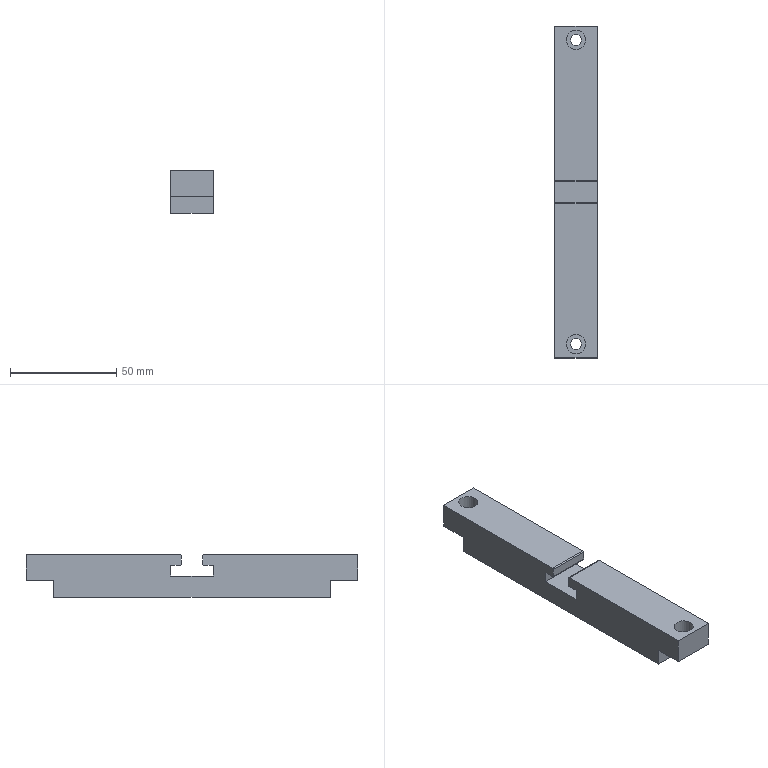Part | STEP file | 200 mesh_id1914 | 1 solid | 28 faces | box 20 x 156 x 20 mm | volume 54101 mm3 | plane 20 | cylinder 8 | commonest cylinder face diameters 1 x4 5.2 x2 9 x2
STEP:
#1=CARTESIAN_POINT('',(-16722.684,-4085.169,68.43));
#2=VERTEX_POINT('',#1);
#3=CARTESIAN_POINT('',(-16722.684,-4098.269,68.43));
#4=VERTEX_POINT('',#3);
#5=CARTESIAN_POINT('',(-16722.684,-4095.569,68.43));
#6=DIRECTION('',(0.,-1.,0.));
#7=VECTOR('',#6,1.);
#8=LINE('',#5,#7);
#9=EDGE_CURVE('',#2,#4,#8,.T.);
#10=ORIENTED_EDGE('',*,*,#9,.F.);
#11=CARTESIAN_POINT('',(-16722.684,-4085.169,60.43));
#12=VERTEX_POINT('',#11);
#13=CARTESIAN_POINT('',(-16722.684,-4085.169,68.63));
#14=DIRECTION('',(0.,0.,-1.));
#15=VECTOR('',#14,1.);
#16=LINE('',#13,#15);
#17=EDGE_CURVE('',#2,#12,#16,.T.);
#18=ORIENTED_EDGE('',*,*,#17,.T.);
#19=CARTESIAN_POINT('',(-16722.684,-3955.369,60.43));
#20=VERTEX_POINT('',#19);
#21=CARTESIAN_POINT('',(-16722.684,-4095.269,60.43));
#22=DIRECTION('',(0.,1.,0.));
#23=VECTOR('',#22,1.);
#24=LINE('',#21,#23);
#25=EDGE_CURVE('',#12,#20,#24,.T.);
#26=ORIENTED_EDGE('',*,*,#25,.T.);
#27=CARTESIAN_POINT('',(-16722.684,-3955.369,68.43));
#28=VERTEX_POINT('',#27);
#29=CARTESIAN_POINT('',(-16722.684,-3955.369,68.63));
#30=DIRECTION('',(0.,0.,1.));
#31=VECTOR('',#30,1.);
#32=LINE('',#29,#31);
#33=EDGE_CURVE('',#20,#28,#32,.T.);
#34=ORIENTED_EDGE('',*,*,#33,.T.);
#35=CARTESIAN_POINT('',(-16722.684,-3942.269,68.43));
#36=VERTEX_POINT('',#35);
#37=CARTESIAN_POINT('',(-16722.684,-3955.369,68.43));
#38=DIRECTION('',(0.,1.,0.));
#39=VECTOR('',#38,1.);
#40=LINE('',#37,#39);
#41=EDGE_CURVE('',#28,#36,#40,.T.);
#42=ORIENTED_EDGE('',*,*,#41,.T.);
#43=CARTESIAN_POINT('',(-16722.684,-3942.269,80.43));
#44=VERTEX_POINT('',#43);
#45=CARTESIAN_POINT('',(-16722.684,-3942.269,60.186));
#46=DIRECTION('',(0.,0.,1.));
#47=VECTOR('',#46,1.);
#48=LINE('',#45,#47);
#49=EDGE_CURVE('',#36,#44,#48,.T.);
#50=ORIENTED_EDGE('',*,*,#49,.T.);
#51=CARTESIAN_POINT('',(-16722.684,-4014.769,80.43));
#52=VERTEX_POINT('',#51);
#53=CARTESIAN_POINT('',(-16722.684,-4095.269,80.43));
#54=DIRECTION('',(0.,1.,0.));
#55=VECTOR('',#54,1.);
#56=LINE('',#53,#55);
#57=EDGE_CURVE('',#52,#44,#56,.T.);
#58=ORIENTED_EDGE('',*,*,#57,.F.);
#59=CARTESIAN_POINT('',(-16722.684,-4015.269,79.93));
#60=VERTEX_POINT('',#59);
#61=CARTESIAN_POINT('',(-16722.684,-4014.769,79.93));
#62=DIRECTION('',(1.,0.,0.));
#63=DIRECTION('',(0.,1.,0.));
#64=AXIS2_PLACEMENT_3D('',#61,#62,#63);
#65=CIRCLE('',#64,0.5);
#66=EDGE_CURVE('',#52,#60,#65,.T.);
#67=ORIENTED_EDGE('',*,*,#66,.T.);
#68=CARTESIAN_POINT('',(-16722.684,-4015.269,75.93));
#69=VERTEX_POINT('',#68);
#70=CARTESIAN_POINT('',(-16722.684,-4015.269,80.43));
#71=DIRECTION('',(0.,0.,-1.));
#72=VECTOR('',#71,1.);
#73=LINE('',#70,#72);
#74=EDGE_CURVE('',#60,#69,#73,.T.);
#75=ORIENTED_EDGE('',*,*,#74,.T.);
#76=CARTESIAN_POINT('',(-16722.684,-4014.769,75.43));
#77=VERTEX_POINT('',#76);
#78=CARTESIAN_POINT('',(-16722.684,-4014.769,75.93));
#79=DIRECTION('',(1.,0.,0.));
#80=DIRECTION('',(0.,1.,0.));
#81=AXIS2_PLACEMENT_3D('',#78,#79,#80);
#82=CIRCLE('',#81,0.5);
#83=EDGE_CURVE('',#69,#77,#82,.T.);
#84=ORIENTED_EDGE('',*,*,#83,.T.);
#85=CARTESIAN_POINT('',(-16722.684,-4010.269,75.43));
#86=VERTEX_POINT('',#85);
#87=CARTESIAN_POINT('',(-16722.684,-4015.269,75.43));
#88=DIRECTION('',(0.,1.,0.));
#89=VECTOR('',#88,1.);
#90=LINE('',#87,#89);
#91=EDGE_CURVE('',#77,#86,#90,.T.);
#92=ORIENTED_EDGE('',*,*,#91,.T.);
#93=CARTESIAN_POINT('',(-16722.684,-4010.269,70.43));
#94=VERTEX_POINT('',#93);
#95=CARTESIAN_POINT('',(-16722.684,-4010.269,75.43));
#96=DIRECTION('',(0.,0.,-1.));
#97=VECTOR('',#96,1.);
#98=LINE('',#95,#97);
#99=EDGE_CURVE('',#86,#94,#98,.T.);
#100=ORIENTED_EDGE('',*,*,#99,.T.);
#101=CARTESIAN_POINT('',(-16722.684,-4030.269,70.43));
#102=VERTEX_POINT('',#101);
#103=CARTESIAN_POINT('',(-16722.684,-4010.269,70.43));
#104=DIRECTION('',(0.,-1.,0.));
#105=VECTOR('',#104,1.);
#106=LINE('',#103,#105);
#107=EDGE_CURVE('',#94,#102,#106,.T.);
#108=ORIENTED_EDGE('',*,*,#107,.T.);
#109=CARTESIAN_POINT('',(-16722.684,-4030.269,75.43));
#110=VERTEX_POINT('',#109);
#111=CARTESIAN_POINT('',(-16722.684,-4030.269,70.43));
#112=DIRECTION('',(0.,0.,1.));
#113=VECTOR('',#112,1.);
#114=LINE('',#111,#113);
#115=EDGE_CURVE('',#102,#110,#114,.T.);
#116=ORIENTED_EDGE('',*,*,#115,.T.);
#117=CARTESIAN_POINT('',(-16722.684,-4025.769,75.43));
#118=VERTEX_POINT('',#117);
#119=CARTESIAN_POINT('',(-16722.684,-4030.269,75.43));
#120=DIRECTION('',(0.,1.,0.));
#121=VECTOR('',#120,1.);
#122=LINE('',#119,#121);
#123=EDGE_CURVE('',#110,#118,#122,.T.);
#124=ORIENTED_EDGE('',*,*,#123,.T.);
#125=CARTESIAN_POINT('',(-16722.684,-4025.269,75.93));
#126=VERTEX_POINT('',#125);
#127=CARTESIAN_POINT('',(-16722.684,-4025.769,75.93));
#128=DIRECTION('',(1.,0.,0.));
#129=DIRECTION('',(0.,1.,0.));
#130=AXIS2_PLACEMENT_3D('',#127,#128,#129);
#131=CIRCLE('',#130,0.5);
#132=EDGE_CURVE('',#118,#126,#131,.T.);
#133=ORIENTED_EDGE('',*,*,#132,.T.);
#134=CARTESIAN_POINT('',(-16722.684,-4025.269,79.93));
#135=VERTEX_POINT('',#134);
#136=CARTESIAN_POINT('',(-16722.684,-4025.269,75.43));
#137=DIRECTION('',(0.,0.,1.));
#138=VECTOR('',#137,1.);
#139=LINE('',#136,#138);
#140=EDGE_CURVE('',#126,#135,#139,.T.);
#141=ORIENTED_EDGE('',*,*,#140,.T.);
#142=CARTESIAN_POINT('',(-16722.684,-4025.769,80.43));
#143=VERTEX_POINT('',#142);
#144=CARTESIAN_POINT('',(-16722.684,-4025.769,79.93));
#145=DIRECTION('',(1.,0.,0.));
#146=DIRECTION('',(0.,1.,0.));
#147=AXIS2_PLACEMENT_3D('',#144,#145,#146);
#148=CIRCLE('',#147,0.5);
#149=EDGE_CURVE('',#135,#143,#148,.T.);
#150=ORIENTED_EDGE('',*,*,#149,.T.);
#151=CARTESIAN_POINT('',(-16722.684,-4098.269,80.43));
#152=VERTEX_POINT('',#151);
#153=CARTESIAN_POINT('',(-16722.684,-4095.269,80.43));
#154=DIRECTION('',(0.,1.,0.));
#155=VECTOR('',#154,1.);
#156=LINE('',#153,#155);
#157=EDGE_CURVE('',#152,#143,#156,.T.);
#158=ORIENTED_EDGE('',*,*,#157,.F.);
#159=CARTESIAN_POINT('',(-16722.684,-4098.269,60.186));
#160=DIRECTION('',(0.,0.,1.));
#161=VECTOR('',#160,1.);
#162=LINE('',#159,#161);
#163=EDGE_CURVE('',#4,#152,#162,.T.);
#164=ORIENTED_EDGE('',*,*,#163,.F.);
#165=EDGE_LOOP('',(#10,#18,#26,#34,#42,#50,#58,#67,#75,#84,#92,#100,#108,#116,#124,#133,#141,#150,#158,#164));
#166=FACE_OUTER_BOUND('',#165,.T.);
#167=CARTESIAN_POINT('',(-16722.684,-4095.269,60.186));
#168=DIRECTION('',(1.,0.,0.));
#169=DIRECTION('',(0.,-1.,0.));
#170=AXIS2_PLACEMENT_3D('',#167,#168,#169);
#171=PLANE('',#170);
#172=ADVANCED_FACE('',(#166),#171,.T.);
#173=CARTESIAN_POINT('',(-16742.684,-4085.169,60.43));
#174=VERTEX_POINT('',#173);
#175=CARTESIAN_POINT('',(-16742.684,-4085.169,68.43));
#176=VERTEX_POINT('',#175);
#177=CARTESIAN_POINT('',(-16742.684,-4085.169,68.63));
#178=DIRECTION('',(0.,0.,1.));
#179=VECTOR('',#178,1.);
#180=LINE('',#177,#179);
#181=EDGE_CURVE('',#174,#176,#180,.T.);
#182=ORIENTED_EDGE('',*,*,#181,.T.);
#183=CARTESIAN_POINT('',(-16742.684,-4098.269,68.43));
#184=VERTEX_POINT('',#183);
#185=CARTESIAN_POINT('',(-16742.684,-3945.269,68.43));
#186=DIRECTION('',(0.,-1.,0.));
#187=VECTOR('',#186,1.);
#188=LINE('',#185,#187);
#189=EDGE_CURVE('',#176,#184,#188,.T.);
#190=ORIENTED_EDGE('',*,*,#189,.T.);
#191=CARTESIAN_POINT('',(-16742.684,-4098.269,80.43));
#192=VERTEX_POINT('',#191);
#193=CARTESIAN_POINT('',(-16742.684,-4098.269,60.186));
#194=DIRECTION('',(0.,0.,1.));
#195=VECTOR('',#194,1.);
#196=LINE('',#193,#195);
#197=EDGE_CURVE('',#184,#192,#196,.T.);
#198=ORIENTED_EDGE('',*,*,#197,.T.);
#199=CARTESIAN_POINT('',(-16742.684,-4025.769,80.43));
#200=VERTEX_POINT('',#199);
#201=CARTESIAN_POINT('',(-16742.684,-3945.269,80.43));
#202=DIRECTION('',(0.,-1.,0.));
#203=VECTOR('',#202,1.);
#204=LINE('',#201,#203);
#205=EDGE_CURVE('',#200,#192,#204,.T.);
#206=ORIENTED_EDGE('',*,*,#205,.F.);
#207=CARTESIAN_POINT('',(-16742.684,-4025.269,79.93));
#208=VERTEX_POINT('',#207);
#209=CARTESIAN_POINT('',(-16742.684,-4025.769,79.93));
#210=DIRECTION('',(-1.,0.,0.));
#211=DIRECTION('',(0.,-1.,0.));
#212=AXIS2_PLACEMENT_3D('',#209,#210,#211);
#213=CIRCLE('',#212,0.5);
#214=EDGE_CURVE('',#200,#208,#213,.T.);
#215=ORIENTED_EDGE('',*,*,#214,.T.);
#216=CARTESIAN_POINT('',(-16742.684,-4025.269,75.93));
#217=VERTEX_POINT('',#216);
#218=CARTESIAN_POINT('',(-16742.684,-4025.269,75.43));
#219=DIRECTION('',(0.,0.,-1.));
#220=VECTOR('',#219,1.);
#221=LINE('',#218,#220);
#222=EDGE_CURVE('',#208,#217,#221,.T.);
#223=ORIENTED_EDGE('',*,*,#222,.T.);
#224=CARTESIAN_POINT('',(-16742.684,-4025.769,75.43));
#225=VERTEX_POINT('',#224);
#226=CARTESIAN_POINT('',(-16742.684,-4025.769,75.93));
#227=DIRECTION('',(-1.,0.,0.));
#228=DIRECTION('',(0.,-1.,0.));
#229=AXIS2_PLACEMENT_3D('',#226,#227,#228);
#230=CIRCLE('',#229,0.5);
#231=EDGE_CURVE('',#217,#225,#230,.T.);
#232=ORIENTED_EDGE('',*,*,#231,.T.);
#233=CARTESIAN_POINT('',(-16742.684,-4030.269,75.43));
#234=VERTEX_POINT('',#233);
#235=CARTESIAN_POINT('',(-16742.684,-4030.269,75.43));
#236=DIRECTION('',(0.,-1.,0.));
#237=VECTOR('',#236,1.);
#238=LINE('',#235,#237);
#239=EDGE_CURVE('',#225,#234,#238,.T.);
#240=ORIENTED_EDGE('',*,*,#239,.T.);
#241=CARTESIAN_POINT('',(-16742.684,-4030.269,70.43));
#242=VERTEX_POINT('',#241);
#243=CARTESIAN_POINT('',(-16742.684,-4030.269,70.43));
#244=DIRECTION('',(0.,0.,-1.));
#245=VECTOR('',#244,1.);
#246=LINE('',#243,#245);
#247=EDGE_CURVE('',#234,#242,#246,.T.);
#248=ORIENTED_EDGE('',*,*,#247,.T.);
#249=CARTESIAN_POINT('',(-16742.684,-4010.269,70.43));
#250=VERTEX_POINT('',#249);
#251=CARTESIAN_POINT('',(-16742.684,-4010.269,70.43));
#252=DIRECTION('',(0.,1.,0.));
#253=VECTOR('',#252,1.);
#254=LINE('',#251,#253);
#255=EDGE_CURVE('',#242,#250,#254,.T.);
#256=ORIENTED_EDGE('',*,*,#255,.T.);
#257=CARTESIAN_POINT('',(-16742.684,-4010.269,75.43));
#258=VERTEX_POINT('',#257);
#259=CARTESIAN_POINT('',(-16742.684,-4010.269,75.43));
#260=DIRECTION('',(0.,0.,1.));
#261=VECTOR('',#260,1.);
#262=LINE('',#259,#261);
#263=EDGE_CURVE('',#250,#258,#262,.T.);
#264=ORIENTED_EDGE('',*,*,#263,.T.);
#265=CARTESIAN_POINT('',(-16742.684,-4014.769,75.43));
#266=VERTEX_POINT('',#265);
#267=CARTESIAN_POINT('',(-16742.684,-4015.269,75.43));
#268=DIRECTION('',(0.,-1.,0.));
#269=VECTOR('',#268,1.);
#270=LINE('',#267,#269);
#271=EDGE_CURVE('',#258,#266,#270,.T.);
#272=ORIENTED_EDGE('',*,*,#271,.T.);
#273=CARTESIAN_POINT('',(-16742.684,-4015.269,75.93));
#274=VERTEX_POINT('',#273);
#275=CARTESIAN_POINT('',(-16742.684,-4014.769,75.93));
#276=DIRECTION('',(-1.,0.,0.));
#277=DIRECTION('',(0.,-1.,0.));
#278=AXIS2_PLACEMENT_3D('',#275,#276,#277);
#279=CIRCLE('',#278,0.5);
#280=EDGE_CURVE('',#266,#274,#279,.T.);
#281=ORIENTED_EDGE('',*,*,#280,.T.);
#282=CARTESIAN_POINT('',(-16742.684,-4015.269,79.93));
#283=VERTEX_POINT('',#282);
#284=CARTESIAN_POINT('',(-16742.684,-4015.269,80.43));
#285=DIRECTION('',(0.,0.,1.));
#286=VECTOR('',#285,1.);
#287=LINE('',#284,#286);
#288=EDGE_CURVE('',#274,#283,#287,.T.);
#289=ORIENTED_EDGE('',*,*,#288,.T.);
#290=CARTESIAN_POINT('',(-16742.684,-4014.769,80.43));
#291=VERTEX_POINT('',#290);
#292=CARTESIAN_POINT('',(-16742.684,-4014.769,79.93));
#293=DIRECTION('',(-1.,0.,0.));
#294=DIRECTION('',(0.,-1.,0.));
#295=AXIS2_PLACEMENT_3D('',#292,#293,#294);
#296=CIRCLE('',#295,0.5);
#297=EDGE_CURVE('',#283,#291,#296,.T.);
#298=ORIENTED_EDGE('',*,*,#297,.T.);
#299=CARTESIAN_POINT('',(-16742.684,-3942.269,80.43));
#300=VERTEX_POINT('',#299);
#301=CARTESIAN_POINT('',(-16742.684,-3945.269,80.43));
#302=DIRECTION('',(0.,-1.,0.));
#303=VECTOR('',#302,1.);
#304=LINE('',#301,#303);
#305=EDGE_CURVE('',#300,#291,#304,.T.);
#306=ORIENTED_EDGE('',*,*,#305,.F.);
#307=CARTESIAN_POINT('',(-16742.684,-3942.269,68.43));
#308=VERTEX_POINT('',#307);
#309=CARTESIAN_POINT('',(-16742.684,-3942.269,60.186));
#310=DIRECTION('',(0.,0.,1.));
#311=VECTOR('',#310,1.);
#312=LINE('',#309,#311);
#313=EDGE_CURVE('',#308,#300,#312,.T.);
#314=ORIENTED_EDGE('',*,*,#313,.F.);
#315=CARTESIAN_POINT('',(-16742.684,-3955.369,68.43));
#316=VERTEX_POINT('',#315);
#317=CARTESIAN_POINT('',(-16742.684,-3945.269,68.43));
#318=DIRECTION('',(0.,1.,0.));
#319=VECTOR('',#318,1.);
#320=LINE('',#317,#319);
#321=EDGE_CURVE('',#316,#308,#320,.T.);
#322=ORIENTED_EDGE('',*,*,#321,.F.);
#323=CARTESIAN_POINT('',(-16742.684,-3955.369,60.43));
#324=VERTEX_POINT('',#323);
#325=CARTESIAN_POINT('',(-16742.684,-3955.369,68.63));
#326=DIRECTION('',(0.,0.,-1.));
#327=VECTOR('',#326,1.);
#328=LINE('',#325,#327);
#329=EDGE_CURVE('',#316,#324,#328,.T.);
#330=ORIENTED_EDGE('',*,*,#329,.T.);
#331=CARTESIAN_POINT('',(-16742.684,-3945.269,60.43));
#332=DIRECTION('',(0.,-1.,0.));
#333=VECTOR('',#332,1.);
#334=LINE('',#331,#333);
#335=EDGE_CURVE('',#324,#174,#334,.T.);
#336=ORIENTED_EDGE('',*,*,#335,.T.);
#337=EDGE_LOOP('',(#182,#190,#198,#206,#215,#223,#232,#240,#248,#256,#264,#272,#281,#289,#298,#306,#314,#322,#330,#336));
#338=FACE_OUTER_BOUND('',#337,.T.);
#339=CARTESIAN_POINT('',(-16742.684,-3945.269,60.186));
#340=DIRECTION('',(-1.,0.,0.));
#341=DIRECTION('',(0.,1.,0.));
#342=AXIS2_PLACEMENT_3D('',#339,#340,#341);
#343=PLANE('',#342);
#344=ADVANCED_FACE('',(#338),#343,.T.);
#345=CARTESIAN_POINT('',(-16737.184,-4091.769,80.43));
#346=VERTEX_POINT('',#345);
#347=CARTESIAN_POINT('',(-16732.684,-4091.769,80.43));
#348=DIRECTION('',(0.,0.,-1.));
#349=DIRECTION('',(-1.,0.,0.));
#350=AXIS2_PLACEMENT_3D('',#347,#348,#349);
#351=CIRCLE('',#350,4.5);
#352=EDGE_CURVE('',#346,#346,#351,.T.);
#353=ORIENTED_EDGE('',*,*,#352,.T.);
#354=EDGE_LOOP('',(#353));
#355=FACE_BOUND('',#354,.T.);
#356=ORIENTED_EDGE('',*,*,#157,.T.);
#357=CARTESIAN_POINT('',(-16732.684,-4025.769,80.43));
#358=DIRECTION('',(-1.,0.,0.));
#359=VECTOR('',#358,1.);
#360=LINE('',#357,#359);
#361=EDGE_CURVE('',#143,#200,#360,.T.);
#362=ORIENTED_EDGE('',*,*,#361,.T.);
#363=ORIENTED_EDGE('',*,*,#205,.T.);
#364=CARTESIAN_POINT('',(-16739.684,-4098.269,80.43));
#365=DIRECTION('',(1.,0.,0.));
#366=VECTOR('',#365,1.);
#367=LINE('',#364,#366);
#368=EDGE_CURVE('',#192,#152,#367,.T.);
#369=ORIENTED_EDGE('',*,*,#368,.T.);
#370=EDGE_LOOP('',(#356,#362,#363,#369));
#371=FACE_BOUND('',#370,.T.);
#372=CARTESIAN_POINT('',(-16732.684,-3950.269,80.43));
#373=DIRECTION('',(0.,0.,-1.));
#374=DIRECTION('',(-1.,0.,0.));
#375=AXIS2_PLACEMENT_3D('',#372,#373,#374);
#376=PLANE('',#375);
#377=ADVANCED_FACE('',(#355,#371),#376,.F.);
#378=ORIENTED_EDGE('',*,*,#49,.F.);
#379=CARTESIAN_POINT('',(-16725.684,-3942.269,68.43));
#380=DIRECTION('',(-1.,0.,0.));
#381=VECTOR('',#380,1.);
#382=LINE('',#379,#381);
#383=EDGE_CURVE('',#36,#308,#382,.T.);
#384=ORIENTED_EDGE('',*,*,#383,.T.);
#385=ORIENTED_EDGE('',*,*,#313,.T.);
#386=CARTESIAN_POINT('',(-16725.684,-3942.269,80.43));
#387=DIRECTION('',(-1.,0.,0.));
#388=VECTOR('',#387,1.);
#389=LINE('',#386,#388);
#390=EDGE_CURVE('',#44,#300,#389,.T.);
#391=ORIENTED_EDGE('',*,*,#390,.F.);
#392=EDGE_LOOP('',(#378,#384,#385,#391));
#393=FACE_OUTER_BOUND('',#392,.T.);
#394=CARTESIAN_POINT('',(-16725.684,-3942.269,60.186));
#395=DIRECTION('',(0.,1.,0.));
#396=DIRECTION('',(0.,0.,-1.));
#397=AXIS2_PLACEMENT_3D('',#394,#395,#396);
#398=PLANE('',#397);
#399=ADVANCED_FACE('',(#393),#398,.T.);
#400=CARTESIAN_POINT('',(-16725.684,-4085.169,60.43));
#401=DIRECTION('',(1.,0.,0.));
#402=VECTOR('',#401,1.);
#403=LINE('',#400,#402);
#404=EDGE_CURVE('',#174,#12,#403,.T.);
#405=ORIENTED_EDGE('',*,*,#404,.F.);
#406=ORIENTED_EDGE('',*,*,#335,.F.);
#407=CARTESIAN_POINT('',(-16725.684,-3955.369,60.43));
#408=DIRECTION('',(-1.,0.,0.));
#409=VECTOR('',#408,1.);
#410=LINE('',#407,#409);
#411=EDGE_CURVE('',#20,#324,#410,.T.);
#412=ORIENTED_EDGE('',*,*,#411,.F.);
#413=ORIENTED_EDGE('',*,*,#25,.F.);
#414=EDGE_LOOP('',(#405,#406,#412,#413));
#415=FACE_OUTER_BOUND('',#414,.T.);
#416=CARTESIAN_POINT('',(-16725.684,-4136.269,60.43));
#417=DIRECTION('',(0.,0.,1.));
#418=DIRECTION('',(0.,1.,0.));
#419=AXIS2_PLACEMENT_3D('',#416,#417,#418);
#420=PLANE('',#419);
#421=ADVANCED_FACE('',(#415),#420,.F.);
#422=CARTESIAN_POINT('',(-16735.284,-4091.769,73.43));
#423=VERTEX_POINT('',#422);
#424=CARTESIAN_POINT('',(-16732.684,-4091.769,73.43));
#425=DIRECTION('',(0.,0.,-1.));
#426=DIRECTION('',(-1.,0.,0.));
#427=AXIS2_PLACEMENT_3D('',#424,#425,#426);
#428=CIRCLE('',#427,2.6);
#429=EDGE_CURVE('',#423,#423,#428,.T.);
#430=ORIENTED_EDGE('',*,*,#429,.F.);
#431=EDGE_LOOP('',(#430));
#432=FACE_BOUND('',#431,.T.);
#433=CARTESIAN_POINT('',(-16730.084,-4091.769,68.43));
#434=VERTEX_POINT('',#433);
#435=CARTESIAN_POINT('',(-16732.684,-4091.769,68.43));
#436=DIRECTION('',(0.,0.,-1.));
#437=DIRECTION('',(1.,0.,0.));
#438=AXIS2_PLACEMENT_3D('',#435,#436,#437);
#439=CIRCLE('',#438,2.6);
#440=EDGE_CURVE('',#434,#434,#439,.T.);
#441=ORIENTED_EDGE('',*,*,#440,.T.);
#442=EDGE_LOOP('',(#441));
#443=FACE_BOUND('',#442,.T.);
#444=CARTESIAN_POINT('',(-16732.684,-4091.769,60.186));
#445=DIRECTION('',(0.,0.,1.));
#446=DIRECTION('',(1.,0.,0.));
#447=AXIS2_PLACEMENT_3D('',#444,#445,#446);
#448=CYLINDRICAL_SURFACE('',#447,2.6);
#449=ADVANCED_FACE('',(#432,#443),#448,.F.);
#450=CARTESIAN_POINT('',(-16735.225,-4098.269,68.43));
#451=DIRECTION('',(-1.,0.,0.));
#452=VECTOR('',#451,1.);
#453=LINE('',#450,#452);
#454=EDGE_CURVE('',#4,#184,#453,.T.);
#455=ORIENTED_EDGE('',*,*,#454,.F.);
#456=ORIENTED_EDGE('',*,*,#163,.T.);
#457=ORIENTED_EDGE('',*,*,#368,.F.);
#458=ORIENTED_EDGE('',*,*,#197,.F.);
#459=EDGE_LOOP('',(#455,#456,#457,#458));
#460=FACE_OUTER_BOUND('',#459,.T.);
#461=CARTESIAN_POINT('',(-16739.684,-4098.269,60.186));
#462=DIRECTION('',(0.,-1.,0.));
#463=DIRECTION('',(0.,0.,1.));
#464=AXIS2_PLACEMENT_3D('',#461,#462,#463);
#465=PLANE('',#464);
#466=ADVANCED_FACE('',(#460),#465,.T.);
#467=CARTESIAN_POINT('',(-16735.284,-3948.769,73.43));
#468=VERTEX_POINT('',#467);
#469=CARTESIAN_POINT('',(-16732.684,-3948.769,73.43));
#470=DIRECTION('',(0.,0.,-1.));
#471=DIRECTION('',(-1.,0.,0.));
#472=AXIS2_PLACEMENT_3D('',#469,#470,#471);
#473=CIRCLE('',#472,2.6);
#474=EDGE_CURVE('',#468,#468,#473,.T.);
#475=ORIENTED_EDGE('',*,*,#474,.F.);
#476=EDGE_LOOP('',(#475));
#477=FACE_BOUND('',#476,.T.);
#478=CARTESIAN_POINT('',(-16730.084,-3948.769,68.43));
#479=VERTEX_POINT('',#478);
#480=CARTESIAN_POINT('',(-16732.684,-3948.769,68.43));
#481=DIRECTION('',(0.,0.,1.));
#482=DIRECTION('',(1.,0.,0.));
#483=AXIS2_PLACEMENT_3D('',#480,#481,#482);
#484=CIRCLE('',#483,2.6);
#485=EDGE_CURVE('',#479,#479,#484,.T.);
#486=ORIENTED_EDGE('',*,*,#485,.F.);
#487=EDGE_LOOP('',(#486));
#488=FACE_BOUND('',#487,.T.);
#489=CARTESIAN_POINT('',(-16732.684,-3948.769,60.186));
#490=DIRECTION('',(0.,0.,1.));
#491=DIRECTION('',(1.,0.,0.));
#492=AXIS2_PLACEMENT_3D('',#489,#490,#491);
#493=CYLINDRICAL_SURFACE('',#492,2.6);
#494=ADVANCED_FACE('',(#477,#488),#493,.F.);
#495=CARTESIAN_POINT('',(-16737.184,-3948.769,80.43));
#496=VERTEX_POINT('',#495);
#497=CARTESIAN_POINT('',(-16732.684,-3948.769,80.43));
#498=DIRECTION('',(0.,0.,-1.));
#499=DIRECTION('',(-1.,0.,0.));
#500=AXIS2_PLACEMENT_3D('',#497,#498,#499);
#501=CIRCLE('',#500,4.5);
#502=EDGE_CURVE('',#496,#496,#501,.T.);
#503=ORIENTED_EDGE('',*,*,#502,.T.);
#504=EDGE_LOOP('',(#503));
#505=FACE_BOUND('',#504,.T.);
#506=ORIENTED_EDGE('',*,*,#305,.T.);
#507=CARTESIAN_POINT('',(-16732.684,-4014.769,80.43));
#508=DIRECTION('',(1.,0.,0.));
#509=VECTOR('',#508,1.);
#510=LINE('',#507,#509);
#511=EDGE_CURVE('',#291,#52,#510,.T.);
#512=ORIENTED_EDGE('',*,*,#511,.T.);
#513=ORIENTED_EDGE('',*,*,#57,.T.);
#514=ORIENTED_EDGE('',*,*,#390,.T.);
#515=EDGE_LOOP('',(#506,#512,#513,#514));
#516=FACE_BOUND('',#515,.T.);
#517=CARTESIAN_POINT('',(-16732.684,-3950.269,80.43));
#518=DIRECTION('',(0.,0.,-1.));
#519=DIRECTION('',(-1.,0.,0.));
#520=AXIS2_PLACEMENT_3D('',#517,#518,#519);
#521=PLANE('',#520);
#522=ADVANCED_FACE('',(#505,#516),#521,.F.);
#523=ORIENTED_EDGE('',*,*,#189,.F.);
#524=CARTESIAN_POINT('',(-16721.684,-4085.169,68.43));
#525=DIRECTION('',(-1.,0.,0.));
#526=VECTOR('',#525,1.);
#527=LINE('',#524,#526);
#528=EDGE_CURVE('',#2,#176,#527,.T.);
#529=ORIENTED_EDGE('',*,*,#528,.F.);
#530=ORIENTED_EDGE('',*,*,#9,.T.);
#531=ORIENTED_EDGE('',*,*,#454,.T.);
#532=EDGE_LOOP('',(#523,#529,#530,#531));
#533=FACE_BOUND('',#532,.T.);
#534=ORIENTED_EDGE('',*,*,#440,.F.);
#535=EDGE_LOOP('',(#534));
#536=FACE_BOUND('',#535,.T.);
#537=CARTESIAN_POINT('',(-16735.225,-4095.569,68.43));
#538=DIRECTION('',(0.,0.,1.));
#539=DIRECTION('',(1.,0.,0.));
#540=AXIS2_PLACEMENT_3D('',#537,#538,#539);
#541=PLANE('',#540);
#542=ADVANCED_FACE('',(#533,#536),#541,.F.);
#543=ORIENTED_EDGE('',*,*,#321,.T.);
#544=ORIENTED_EDGE('',*,*,#383,.F.);
#545=ORIENTED_EDGE('',*,*,#41,.F.);
#546=CARTESIAN_POINT('',(-16725.684,-3955.369,68.43));
#547=DIRECTION('',(1.,0.,0.));
#548=VECTOR('',#547,1.);
#549=LINE('',#546,#548);
#550=EDGE_CURVE('',#316,#28,#549,.T.);
#551=ORIENTED_EDGE('',*,*,#550,.F.);
#552=EDGE_LOOP('',(#543,#544,#545,#551));
#553=FACE_BOUND('',#552,.T.);
#554=ORIENTED_EDGE('',*,*,#485,.T.);
#555=EDGE_LOOP('',(#554));
#556=FACE_BOUND('',#555,.T.);
#557=CARTESIAN_POINT('',(-16725.684,-3955.369,68.43));
#558=DIRECTION('',(0.,0.,1.));
#559=DIRECTION('',(1.,0.,0.));
#560=AXIS2_PLACEMENT_3D('',#557,#558,#559);
#561=PLANE('',#560);
#562=ADVANCED_FACE('',(#553,#556),#561,.F.);
#563=ORIENTED_EDGE('',*,*,#429,.T.);
#564=EDGE_LOOP('',(#563));
#565=FACE_BOUND('',#564,.T.);
#566=CARTESIAN_POINT('',(-16728.184,-4091.769,73.43));
#567=VERTEX_POINT('',#566);
#568=CARTESIAN_POINT('',(-16732.684,-4091.769,73.43));
#569=DIRECTION('',(0.,0.,-1.));
#570=DIRECTION('',(1.,0.,0.));
#571=AXIS2_PLACEMENT_3D('',#568,#569,#570);
#572=CIRCLE('',#571,4.5);
#573=EDGE_CURVE('',#567,#567,#572,.T.);
#574=ORIENTED_EDGE('',*,*,#573,.F.);
#575=EDGE_LOOP('',(#574));
#576=FACE_BOUND('',#575,.T.);
#577=CARTESIAN_POINT('',(-16732.684,-4091.769,73.43));
#578=DIRECTION('',(0.,0.,-1.));
#579=DIRECTION('',(-1.,0.,0.));
#580=AXIS2_PLACEMENT_3D('',#577,#578,#579);
#581=PLANE('',#580);
#582=ADVANCED_FACE('',(#565,#576),#581,.F.);
#583=ORIENTED_EDGE('',*,*,#573,.T.);
#584=EDGE_LOOP('',(#583));
#585=FACE_BOUND('',#584,.T.);
#586=ORIENTED_EDGE('',*,*,#352,.F.);
#587=EDGE_LOOP('',(#586));
#588=FACE_BOUND('',#587,.T.);
#589=CARTESIAN_POINT('',(-16732.684,-4091.769,78.43));
#590=DIRECTION('',(0.,0.,-1.));
#591=DIRECTION('',(1.,0.,0.));
#592=AXIS2_PLACEMENT_3D('',#589,#590,#591);
#593=CYLINDRICAL_SURFACE('',#592,4.5);
#594=ADVANCED_FACE('',(#585,#588),#593,.F.);
#595=ORIENTED_EDGE('',*,*,#474,.T.);
#596=EDGE_LOOP('',(#595));
#597=FACE_BOUND('',#596,.T.);
#598=CARTESIAN_POINT('',(-16728.184,-3948.769,73.43));
#599=VERTEX_POINT('',#598);
#600=CARTESIAN_POINT('',(-16732.684,-3948.769,73.43));
#601=DIRECTION('',(0.,0.,1.));
#602=DIRECTION('',(1.,0.,0.));
#603=AXIS2_PLACEMENT_3D('',#600,#601,#602);
#604=CIRCLE('',#603,4.5);
#605=EDGE_CURVE('',#599,#599,#604,.T.);
#606=ORIENTED_EDGE('',*,*,#605,.T.);
#607=EDGE_LOOP('',(#606));
#608=FACE_BOUND('',#607,.T.);
#609=CARTESIAN_POINT('',(-16732.684,-3948.769,73.43));
#610=DIRECTION('',(0.,0.,-1.));
#611=DIRECTION('',(-1.,0.,0.));
#612=AXIS2_PLACEMENT_3D('',#609,#610,#611);
#613=PLANE('',#612);
#614=ADVANCED_FACE('',(#597,#608),#613,.F.);
#615=ORIENTED_EDGE('',*,*,#605,.F.);
#616=EDGE_LOOP('',(#615));
#617=FACE_BOUND('',#616,.T.);
#618=ORIENTED_EDGE('',*,*,#502,.F.);
#619=EDGE_LOOP('',(#618));
#620=FACE_BOUND('',#619,.T.);
#621=CARTESIAN_POINT('',(-16732.684,-3948.769,78.43));
#622=DIRECTION('',(0.,0.,-1.));
#623=DIRECTION('',(1.,0.,0.));
#624=AXIS2_PLACEMENT_3D('',#621,#622,#623);
#625=CYLINDRICAL_SURFACE('',#624,4.5);
#626=ADVANCED_FACE('',(#617,#620),#625,.F.);
#627=ORIENTED_EDGE('',*,*,#288,.F.);
#628=CARTESIAN_POINT('',(-16718.684,-4015.269,75.93));
#629=DIRECTION('',(1.,0.,0.));
#630=VECTOR('',#629,1.);
#631=LINE('',#628,#630);
#632=EDGE_CURVE('',#274,#69,#631,.T.);
#633=ORIENTED_EDGE('',*,*,#632,.T.);
#634=ORIENTED_EDGE('',*,*,#74,.F.);
#635=CARTESIAN_POINT('',(-16718.684,-4015.269,79.93));
#636=DIRECTION('',(-1.,0.,0.));
#637=VECTOR('',#636,1.);
#638=LINE('',#635,#637);
#639=EDGE_CURVE('',#60,#283,#638,.T.);
#640=ORIENTED_EDGE('',*,*,#639,.T.);
#641=EDGE_LOOP('',(#627,#633,#634,#640));
#642=FACE_OUTER_BOUND('',#641,.T.);
#643=CARTESIAN_POINT('',(-16718.684,-4015.269,80.43));
#644=DIRECTION('',(0.,1.,0.));
#645=DIRECTION('',(0.,0.,1.));
#646=AXIS2_PLACEMENT_3D('',#643,#644,#645);
#647=PLANE('',#646);
#648=ADVANCED_FACE('',(#642),#647,.F.);
#649=ORIENTED_EDGE('',*,*,#91,.F.);
#650=CARTESIAN_POINT('',(-16718.684,-4014.769,75.43));
#651=DIRECTION('',(-1.,0.,0.));
#652=VECTOR('',#651,1.);
#653=LINE('',#650,#652);
#654=EDGE_CURVE('',#77,#266,#653,.T.);
#655=ORIENTED_EDGE('',*,*,#654,.T.);
#656=ORIENTED_EDGE('',*,*,#271,.F.);
#657=CARTESIAN_POINT('',(-16718.684,-4010.269,75.43));
#658=DIRECTION('',(1.,0.,0.));
#659=VECTOR('',#658,1.);
#660=LINE('',#657,#659);
#661=EDGE_CURVE('',#258,#86,#660,.T.);
#662=ORIENTED_EDGE('',*,*,#661,.T.);
#663=EDGE_LOOP('',(#649,#655,#656,#662));
#664=FACE_OUTER_BOUND('',#663,.T.);
#665=CARTESIAN_POINT('',(-16718.684,-4015.269,75.43));
#666=DIRECTION('',(0.,0.,1.));
#667=DIRECTION('',(1.,0.,0.));
#668=AXIS2_PLACEMENT_3D('',#665,#666,#667);
#669=PLANE('',#668);
#670=ADVANCED_FACE('',(#664),#669,.F.);
#671=CARTESIAN_POINT('',(-16718.684,-4010.269,70.43));
#672=DIRECTION('',(1.,0.,0.));
#673=VECTOR('',#672,1.);
#674=LINE('',#671,#673);
#675=EDGE_CURVE('',#250,#94,#674,.T.);
#676=ORIENTED_EDGE('',*,*,#675,.T.);
#677=ORIENTED_EDGE('',*,*,#99,.F.);
#678=ORIENTED_EDGE('',*,*,#661,.F.);
#679=ORIENTED_EDGE('',*,*,#263,.F.);
#680=EDGE_LOOP('',(#676,#677,#678,#679));
#681=FACE_OUTER_BOUND('',#680,.T.);
#682=CARTESIAN_POINT('',(-16718.684,-4010.269,75.43));
#683=DIRECTION('',(0.,1.,0.));
#684=DIRECTION('',(0.,0.,1.));
#685=AXIS2_PLACEMENT_3D('',#682,#683,#684);
#686=PLANE('',#685);
#687=ADVANCED_FACE('',(#681),#686,.F.);
#688=CARTESIAN_POINT('',(-16718.684,-4030.269,75.43));
#689=DIRECTION('',(1.,0.,0.));
#690=VECTOR('',#689,1.);
#691=LINE('',#688,#690);
#692=EDGE_CURVE('',#234,#110,#691,.T.);
#693=ORIENTED_EDGE('',*,*,#692,.T.);
#694=ORIENTED_EDGE('',*,*,#115,.F.);
#695=CARTESIAN_POINT('',(-16718.684,-4030.269,70.43));
#696=DIRECTION('',(1.,0.,0.));
#697=VECTOR('',#696,1.);
#698=LINE('',#695,#697);
#699=EDGE_CURVE('',#242,#102,#698,.T.);
#700=ORIENTED_EDGE('',*,*,#699,.F.);
#701=ORIENTED_EDGE('',*,*,#247,.F.);
#702=EDGE_LOOP('',(#693,#694,#700,#701));
#703=FACE_OUTER_BOUND('',#702,.T.);
#704=CARTESIAN_POINT('',(-16718.684,-4030.269,70.43));
#705=DIRECTION('',(0.,-1.,0.));
#706=DIRECTION('',(0.,0.,-1.));
#707=AXIS2_PLACEMENT_3D('',#704,#705,#706);
#708=PLANE('',#707);
#709=ADVANCED_FACE('',(#703),#708,.F.);
#710=ORIENTED_EDGE('',*,*,#239,.F.);
#711=CARTESIAN_POINT('',(-16718.684,-4025.769,75.43));
#712=DIRECTION('',(1.,0.,0.));
#713=VECTOR('',#712,1.);
#714=LINE('',#711,#713);
#715=EDGE_CURVE('',#225,#118,#714,.T.);
#716=ORIENTED_EDGE('',*,*,#715,.T.);
#717=ORIENTED_EDGE('',*,*,#123,.F.);
#718=ORIENTED_EDGE('',*,*,#692,.F.);
#719=EDGE_LOOP('',(#710,#716,#717,#718));
#720=FACE_OUTER_BOUND('',#719,.T.);
#721=CARTESIAN_POINT('',(-16718.684,-4030.269,75.43));
#722=DIRECTION('',(0.,0.,1.));
#723=DIRECTION('',(1.,0.,0.));
#724=AXIS2_PLACEMENT_3D('',#721,#722,#723);
#725=PLANE('',#724);
#726=ADVANCED_FACE('',(#720),#725,.F.);
#727=ORIENTED_EDGE('',*,*,#222,.F.);
#728=CARTESIAN_POINT('',(-16718.684,-4025.269,79.93));
#729=DIRECTION('',(1.,0.,0.));
#730=VECTOR('',#729,1.);
#731=LINE('',#728,#730);
#732=EDGE_CURVE('',#208,#135,#731,.T.);
#733=ORIENTED_EDGE('',*,*,#732,.T.);
#734=ORIENTED_EDGE('',*,*,#140,.F.);
#735=CARTESIAN_POINT('',(-16718.684,-4025.269,75.93));
#736=DIRECTION('',(-1.,0.,0.));
#737=VECTOR('',#736,1.);
#738=LINE('',#735,#737);
#739=EDGE_CURVE('',#126,#217,#738,.T.);
#740=ORIENTED_EDGE('',*,*,#739,.T.);
#741=EDGE_LOOP('',(#727,#733,#734,#740));
#742=FACE_OUTER_BOUND('',#741,.T.);
#743=CARTESIAN_POINT('',(-16718.684,-4025.269,75.43));
#744=DIRECTION('',(0.,-1.,0.));
#745=DIRECTION('',(0.,0.,-1.));
#746=AXIS2_PLACEMENT_3D('',#743,#744,#745);
#747=PLANE('',#746);
#748=ADVANCED_FACE('',(#742),#747,.F.);
#749=ORIENTED_EDGE('',*,*,#699,.T.);
#750=ORIENTED_EDGE('',*,*,#107,.F.);
#751=ORIENTED_EDGE('',*,*,#675,.F.);
#752=ORIENTED_EDGE('',*,*,#255,.F.);
#753=EDGE_LOOP('',(#749,#750,#751,#752));
#754=FACE_OUTER_BOUND('',#753,.T.);
#755=CARTESIAN_POINT('',(-16718.684,-4010.269,70.43));
#756=DIRECTION('',(0.,0.,-1.));
#757=DIRECTION('',(-1.,0.,0.));
#758=AXIS2_PLACEMENT_3D('',#755,#756,#757);
#759=PLANE('',#758);
#760=ADVANCED_FACE('',(#754),#759,.F.);
#761=ORIENTED_EDGE('',*,*,#149,.F.);
#762=ORIENTED_EDGE('',*,*,#732,.F.);
#763=ORIENTED_EDGE('',*,*,#214,.F.);
#764=ORIENTED_EDGE('',*,*,#361,.F.);
#765=EDGE_LOOP('',(#761,#762,#763,#764));
#766=FACE_OUTER_BOUND('',#765,.T.);
#767=CARTESIAN_POINT('',(-16732.684,-4025.769,79.93));
#768=DIRECTION('',(-1.,0.,0.));
#769=DIRECTION('',(0.,0.,1.));
#770=AXIS2_PLACEMENT_3D('',#767,#768,#769);
#771=CYLINDRICAL_SURFACE('',#770,0.5);
#772=ADVANCED_FACE('',(#766),#771,.T.);
#773=ORIENTED_EDGE('',*,*,#231,.F.);
#774=ORIENTED_EDGE('',*,*,#739,.F.);
#775=ORIENTED_EDGE('',*,*,#132,.F.);
#776=ORIENTED_EDGE('',*,*,#715,.F.);
#777=EDGE_LOOP('',(#773,#774,#775,#776));
#778=FACE_OUTER_BOUND('',#777,.T.);
#779=CARTESIAN_POINT('',(-16718.684,-4025.769,75.93));
#780=DIRECTION('',(1.,0.,0.));
#781=DIRECTION('',(0.,0.,-1.));
#782=AXIS2_PLACEMENT_3D('',#779,#780,#781);
#783=CYLINDRICAL_SURFACE('',#782,0.5);
#784=ADVANCED_FACE('',(#778),#783,.T.);
#785=ORIENTED_EDGE('',*,*,#280,.F.);
#786=ORIENTED_EDGE('',*,*,#654,.F.);
#787=ORIENTED_EDGE('',*,*,#83,.F.);
#788=ORIENTED_EDGE('',*,*,#632,.F.);
#789=EDGE_LOOP('',(#785,#786,#787,#788));
#790=FACE_OUTER_BOUND('',#789,.T.);
#791=CARTESIAN_POINT('',(-16718.684,-4014.769,75.93));
#792=DIRECTION('',(1.,0.,0.));
#793=DIRECTION('',(0.,0.,-1.));
#794=AXIS2_PLACEMENT_3D('',#791,#792,#793);
#795=CYLINDRICAL_SURFACE('',#794,0.5);
#796=ADVANCED_FACE('',(#790),#795,.T.);
#797=ORIENTED_EDGE('',*,*,#297,.F.);
#798=ORIENTED_EDGE('',*,*,#639,.F.);
#799=ORIENTED_EDGE('',*,*,#66,.F.);
#800=ORIENTED_EDGE('',*,*,#511,.F.);
#801=EDGE_LOOP('',(#797,#798,#799,#800));
#802=FACE_OUTER_BOUND('',#801,.T.);
#803=CARTESIAN_POINT('',(-16732.684,-4014.769,79.93));
#804=DIRECTION('',(1.,0.,0.));
#805=DIRECTION('',(0.,0.,-1.));
#806=AXIS2_PLACEMENT_3D('',#803,#804,#805);
#807=CYLINDRICAL_SURFACE('',#806,0.5);
#808=ADVANCED_FACE('',(#802),#807,.T.);
#809=ORIENTED_EDGE('',*,*,#33,.F.);
#810=ORIENTED_EDGE('',*,*,#411,.T.);
#811=ORIENTED_EDGE('',*,*,#329,.F.);
#812=ORIENTED_EDGE('',*,*,#550,.T.);
#813=EDGE_LOOP('',(#809,#810,#811,#812));
#814=FACE_OUTER_BOUND('',#813,.T.);
#815=CARTESIAN_POINT('',(-16721.684,-3955.369,68.63));
#816=DIRECTION('',(0.,-1.,0.));
#817=DIRECTION('',(0.,0.,-1.));
#818=AXIS2_PLACEMENT_3D('',#815,#816,#817);
#819=PLANE('',#818);
#820=ADVANCED_FACE('',(#814),#819,.F.);
#821=ORIENTED_EDGE('',*,*,#181,.F.);
#822=ORIENTED_EDGE('',*,*,#404,.T.);
#823=ORIENTED_EDGE('',*,*,#17,.F.);
#824=ORIENTED_EDGE('',*,*,#528,.T.);
#825=EDGE_LOOP('',(#821,#822,#823,#824));
#826=FACE_OUTER_BOUND('',#825,.T.);
#827=CARTESIAN_POINT('',(-16721.684,-4085.169,68.63));
#828=DIRECTION('',(0.,1.,0.));
#829=DIRECTION('',(0.,0.,-1.));
#830=AXIS2_PLACEMENT_3D('',#827,#828,#829);
#831=PLANE('',#830);
#832=ADVANCED_FACE('',(#826),#831,.F.);
#833=CLOSED_SHELL('',(#172,#344,#377,#399,#421,#449,#466,#494,#522,#542,#562,#582,#594,#614,#626,#648,#670,#687,#709,#726,#748,#760,#772,#784,#796,#808,#820,#832));
#834=MANIFOLD_SOLID_BREP('',#833);
#835=(LENGTH_UNIT()NAMED_UNIT(*)SI_UNIT(.MILLI.,.METRE.));
#836=UNCERTAINTY_MEASURE_WITH_UNIT(LENGTH_MEASURE(0.00002),#835,'','');
#837=(NAMED_UNIT(*)PLANE_ANGLE_UNIT()SI_UNIT($,.RADIAN.));
#838=PLANE_ANGLE_MEASURE_WITH_UNIT(PLANE_ANGLE_MEASURE(0.01745),#837);
#839=DIMENSIONAL_EXPONENTS(0.,0.,0.,0.,0.,0.,0.);
#840=(CONVERSION_BASED_UNIT('DEGREE',#838)NAMED_UNIT(#839)PLANE_ANGLE_UNIT());
#841=(NAMED_UNIT(*)SI_UNIT($,.STERADIAN.)SOLID_ANGLE_UNIT());
#842=(GEOMETRIC_REPRESENTATION_CONTEXT(3)GLOBAL_UNCERTAINTY_ASSIGNED_CONTEXT((#836))GLOBAL_UNIT_ASSIGNED_CONTEXT((#835,#840,#841))REPRESENTATION_CONTEXT('',''));
#843=ADVANCED_BREP_SHAPE_REPRESENTATION('',(#834),#842);